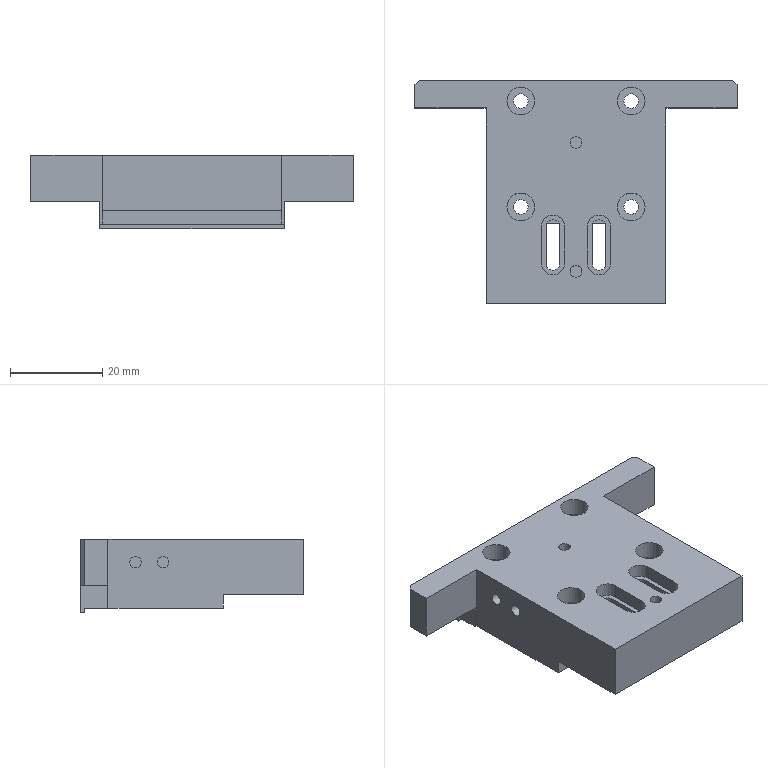Part | 1 solid | 64 faces | box 70 x 48.5 x 16 mm | volume 26355 mm3 | plane 42 | cylinder 22 | commonest cylinder face diameters 2.5 x4 3 x4 3.2 x4 5 x4 6 x4 1.6 x2